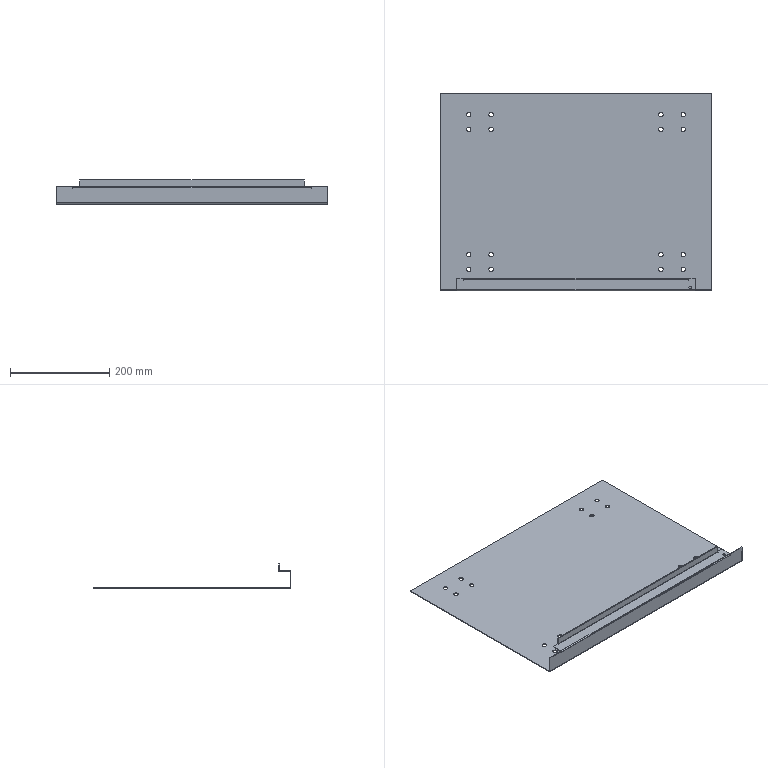Part | SolidWorks | features EdgeFlange 3, ICE 2, MirrorPattern 2, FlatPattern 1, SMBaseFlange 1, SheetMetal 1 | 1 solid | 80 faces | box 547 x 398.5 x 48.5 mm | volume 377197 mm3 | cylinder 40 | plane 40 | commonest cylinder face diameters 9 x32 1.473 x3 4.473 x3 5.5 x2